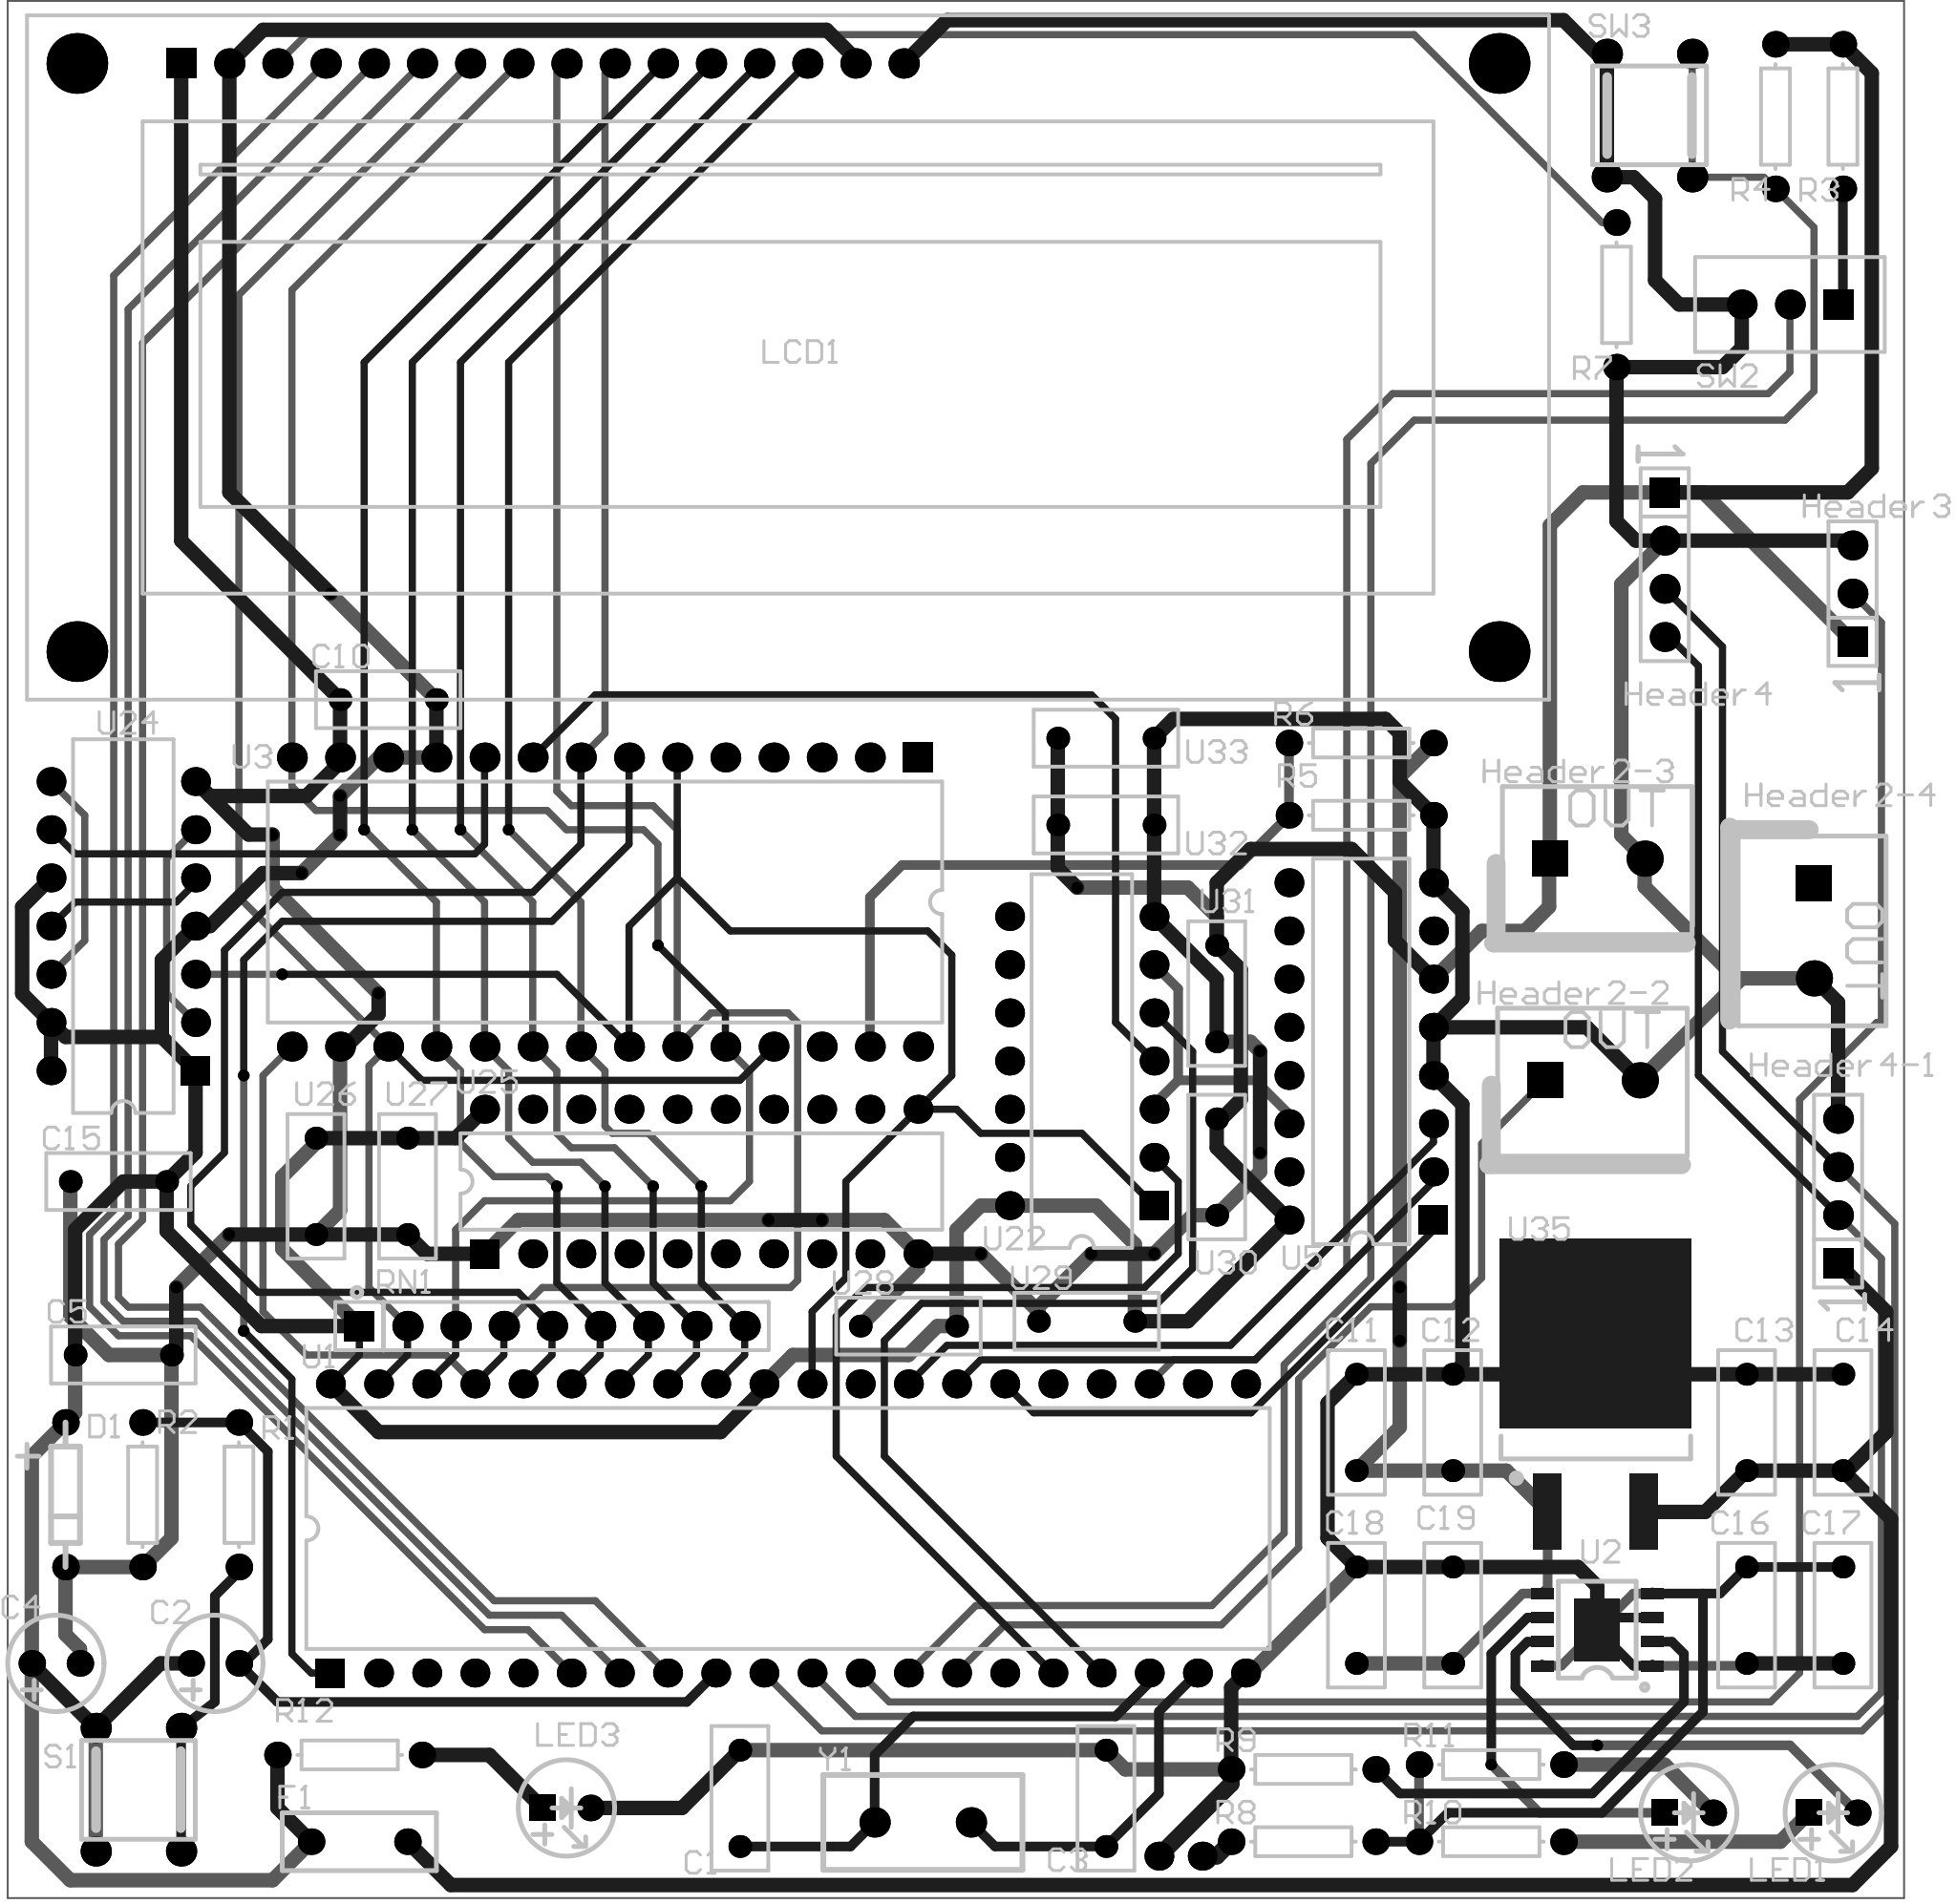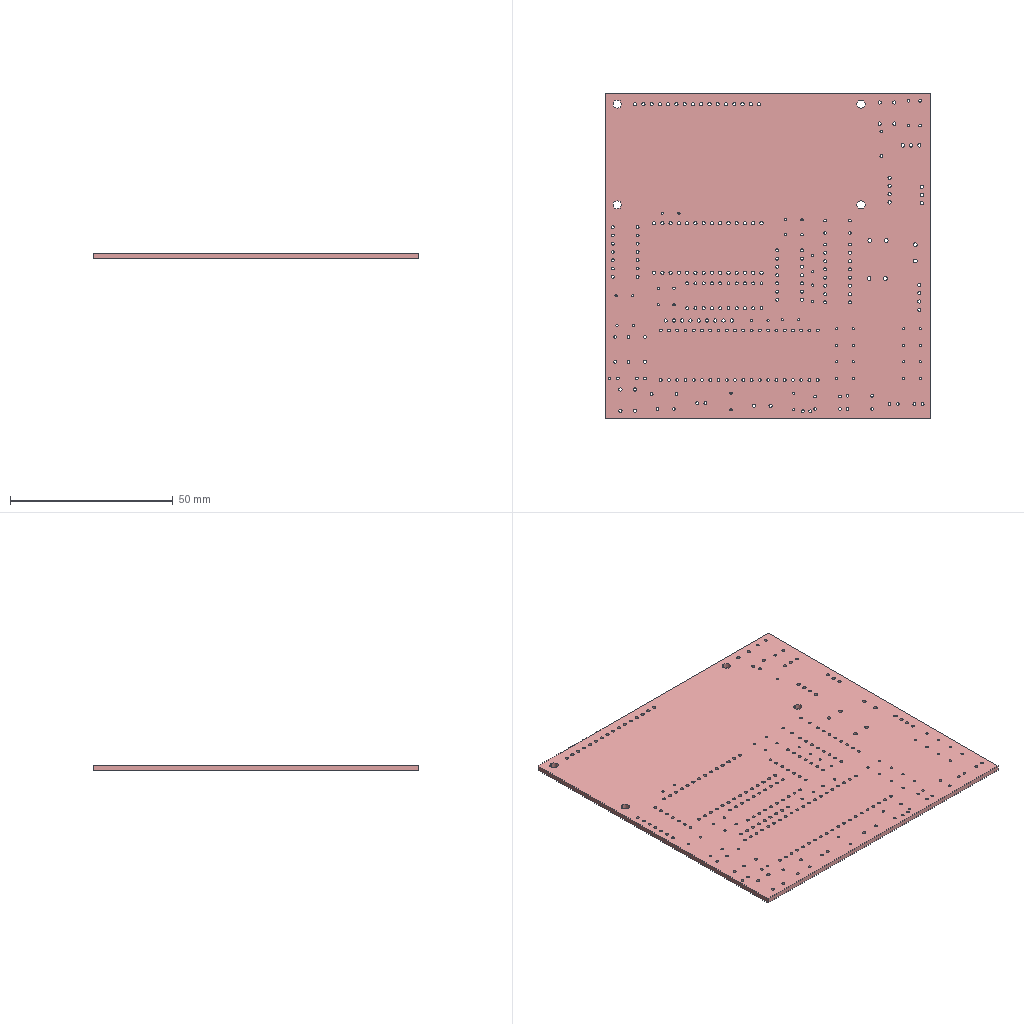Circuit board layout | Altium Designer | box 100 x 100 x 1.6 mm
Layer stack:
# Altium Designer layer stack of  (unit mm; dielectric type: 0 none, 1 core, 2 prepreg, 3 surface material)
index,name,kind,layer,copper_thickness_mm,dielectric_type,dielectric_thickness_mm,dielectric_material,dielectric_constant
0,Top Paste Mask Layer,other,,,,,,
1,Top Silkscreen Layer,other,,,,,,
2,Top Solder Mask Layer,dielectric,,,3,0.01,,3.3
3,Top Layer,copper,Top Layer,0.035,,,,
4,Dielectric1,dielectric,,,3,1.51,FR4,4.5
5,Bottom Layer,copper,Bottom Layer,0.035,,,,
6,Bottom Solder Mask Layer,dielectric,,,3,0.01,,3.3
7,Bottom Silkscreen Layer,other,,,,,,
8,Bottom Paste Mask Layer,other,,,,,,
# drill layer pairs: low layer,high layer
drill_pair,Top Layer,Bottom Layer
Part placement:
Designator,Comment,Layer,Footprint,Center-X(mm),Center-Y(mm),Rotation
U1,STC89C51RC-40I-PDIP40,TopLayer,DIP-40,117.348,95.682,0
Y1,11.059MHz,TopLayer,XTAL-2,124.455,80.189,0
C1,33pF,TopLayer,RAD-0.2,114.808,81.458,90
C3,33pF,TopLayer,RAD-0.2,134.112,81.458,90
C2,10uF,TopLayer,RB1-2,87.122,88.57,90
R1,200Ω,TopLayer,AXIAL-0.3,88.392,97.46,90
R2,10kΩ,TopLayer,AXIAL-0.3,83.312,97.46,270
S1,,TopLayer,RST,83.094,81.914,180
C5,100nF,TopLayer,RAD-0.2,82.296,104.826,0
C4,22uF,TopLayer,RB1-2,78.74,88.57,90
D1,1N5819,TopLayer,DIODE-3,79.248,97.46,180
F1,JK60-050,TopLayer,FUSE-2,94.742,79.172,0
U3,ADC0809CCV/NOPB,TopLayer,DIP-28,107.696,128.702,270
U5,74HC138D,653,TopLayer,DIP-16,147.574,120.828,180
U22,74HC02DRG,TopLayer,DIP-14,132.842,120.32,90
SW2,KH-SS12D01-G3-5.0,TopLayer,RT,170.18,160.198,90
Header4-1,PM254-1-04-W-8.5,TopLayer,CON4,172.72,113.462,90
U24,SN74HC74N,TopLayer,DIP-14,82.296,127.432,90
U25,74HC573D,653,TopLayer,DIP-20,112.776,113.97,0
U26,100nF,TopLayer,RAD-0.2,92.456,113.716,90
U27,100nF,TopLayer,RAD-0.2,97.282,113.716,90
U28,100nF,TopLayer,RAD-0.2,123.698,106.35,0
U29,100nF,TopLayer,RAD-0.2,133.096,106.604,0
U30,100nF,TopLayer,RAD-0.2,139.954,114.732,90
U31,100nF,TopLayer,RAD-0.2,139.954,123.876,90
U32,100nF,TopLayer,RAD-0.2,134.112,132.766,180
U33,100nF,TopLayer,RAD-0.2,134.112,137.338,180
RN1,4.7kΩ,TopLayer,RP,104.902,106.35,0
R3,1kΩ,TopLayer,AXIAL-0.3,172.974,170.104,90
C10,100nF,TopLayer,RAD-0.2,96.266,139.37,0
U35,LM7805S2/TR,TopLayer,TO-263-2_L10.0-W9.1-P5.08-LS15.2-BL,159.945,101.253,0
C11,100nF,TopLayer,RAD-0.2,147.32,101.27,270
C12,100nF,TopLayer,RAD-0.2,152.4,101.27,270
C13,10uF,TopLayer,RAD-0.2,167.894,101.27,270
C14,10uF,TopLayer,RAD-0.2,172.974,101.27,270
SW3,,TopLayer,RST,162.778,170.156,0
R4,10kΩ,TopLayer,AXIAL-0.3,169.418,170.104,90
LED1,204-10SYGD/S530-E3,TopLayer,LED1,172.466,80.696,90
LCD1,LCM1602K-NSW-BBW,TopLayer,LCD1602,117.348,157.404,0
Header4,PM254-1-04-W-8.5,TopLayer,CON4,163.576,146.482,270
R5,10kΩ,TopLayer,AXIAL-0.3,147.574,133.274,180
R6,10kΩ,TopLayer,AXIAL-0.3,147.574,137.084,0
C15,100nF,TopLayer,RAD-0.2,82.042,113.97,0
R7,3.5kΩ,TopLayer,AXIAL-0.3,161.036,160.706,90
Header2-2,XY-XHB2.54-2A21,TopLayer,CON2-5,159.766,119.304,0
Header3,PM254V-11-03-H85,TopLayer,CON3,173.482,144.958,0
Header2-3,XY-XHB2.54-2A21,TopLayer,CON2-5,160.02,130.988,0
Header2-4,XY-XHB2.54-2A21,TopLayer,CON2-5,171.45,127.178,270
C16,10uF,TopLayer,RAD-0.2,167.894,91.11,90
C17,100nF,TopLayer,RAD-0.2,172.974,91.11,90
LED2,333-2SYGD/S530-E2-L,TopLayer,LED1,164.846,80.696,90
R8,250mΩ,TopLayer,AXIAL-0.3,144.526,79.172,0
R9,1.2kΩ,TopLayer,AXIAL-0.3,144.526,82.982,0
R10,2kΩ,TopLayer,AXIAL-0.3,154.432,79.172,0
R11,2kΩ,TopLayer,AXIAL-0.3,154.432,83.236,0
C18,10uF,TopLayer,RAD-0.2,147.32,91.11,270
C19,100nF,TopLayer,RAD-0.2,152.4,91.11,270
R12,1kΩ,TopLayer,AXIAL-0.3,94.234,83.744,180
U2,TP4056-42-ESOP8,TopLayer,ESOP-8_L4.9-W3.9-P1.27-LS6.0-BL-EP,160.02,90.348,90
LED3,204-10SYGD/S530-E3,TopLayer,LED1,105.664,80.95,90
Pad and via stacks:
# Altium Designer via and pad stacks of  (unit mm). Each distinct definition once, with the count of objects using it.
# via: kind,start_layer,end_layer,hole_mm,diameter_mm,mode(0 simple;1 top-mid-bottom;2 full stack),diameter_per_layer,count,example_net
# pad: kind,layer,hole_mm,hole_type(0 round;1 square;2 slot),plating,top_size,top_shape(1 round;2 rect;3 octagon;9 rounded rect),mid_size,bottom_size,mode,footprint,size_per_layer,count,example
pad,Multi-Layer,0.9144,0,plated,1.524x1.524,1,1.524x1.524,1.524x1.524,0,,,2,41
pad,Multi-Layer,0.889,0,plated,1.524x1.524,1,1.524x1.524,1.524x1.524,0,DIP-40,,39,U1.18
pad,Multi-Layer,0.889,0,plated,1.524x1.524,2,1.524x1.524,1.524x1.524,0,DIP-40,,1,U1.1
pad,Multi-Layer,1,0,plated,1.6x1.6,1,1.6x1.6,1.6x1.6,0,XTAL-2,,2,Y1.1
pad,Multi-Layer,0.7,0,plated,1.2x1.2,1,1.2x1.2,1.2x1.2,0,RAD-0.2,,42,C1.2
pad,Multi-Layer,0.85,0,plated,1.4x1.4,1,1.4x1.4,1.4x1.4,0,RB1-2,,4,C2.2
pad,Multi-Layer,0.85,0,plated,1.4x1.4,1,1.4x1.4,1.4x1.4,0,AXIAL-0.3,,24,R1.2
pad,Multi-Layer,1,0,plated,1.6x1.6,1,1.6x1.6,1.6x1.6,0,RST,,8,S1.1
pad,Multi-Layer,0.85,0,plated,1.4x1.4,1,1.4x1.4,1.4x1.4,0,DIODE-3,,2,D1.2
pad,Multi-Layer,0.85,0,plated,1.4x1.4,1,1.4x1.4,1.4x1.4,0,FUSE-2,,2,F1.1
pad,Multi-Layer,1.016,0,plated,1.575x1.575,1,1.575x1.575,1.575x1.575,0,DIP-28,,27,U3.2
pad,Multi-Layer,1.016,0,plated,1.575x1.575,2,1.575x1.575,1.575x1.575,0,DIP-28,,1,U3.1
pad,Multi-Layer,0.889,0,plated,1.524x1.524,1,1.524x1.524,1.524x1.524,0,DIP-16,,15,U5.12
pad,Multi-Layer,0.889,0,plated,1.524x1.524,2,1.524x1.524,1.524x1.524,0,DIP-16,,1,U5.1
pad,Multi-Layer,0.889,0,plated,1.524x1.524,1,1.524x1.524,1.524x1.524,0,DIP-14,,26,U22.11
pad,Multi-Layer,0.889,0,plated,1.524x1.524,2,1.524x1.524,1.524x1.524,0,DIP-14,,2,U22.1
pad,Multi-Layer,1.016,0,plated,1.575x1.575,2,1.575x1.575,1.575x1.575,0,RT,,1,SW2.1
pad,Multi-Layer,1.016,0,plated,1.575x1.575,1,1.575x1.575,1.575x1.575,0,RT,,2,SW2.2
pad,Multi-Layer,1.016,0,plated,1.575x1.575,1,1.575x1.575,1.575x1.575,0,CON4,,6,Header4-1.4
pad,Multi-Layer,1.016,0,plated,1.575x1.575,2,1.575x1.575,1.575x1.575,0,CON4,,2,Header4-1.1
pad,Multi-Layer,0.889,0,plated,1.524x1.524,2,1.524x1.524,1.524x1.524,0,DIP-20,,1,U25.1
pad,Multi-Layer,0.889,0,plated,1.524x1.524,1,1.524x1.524,1.524x1.524,0,DIP-20,,19,U25.2
pad,Multi-Layer,1,0,plated,1.6x1.6,2,1.6x1.6,1.6x1.6,0,RP,,1,RN1.1
pad,Multi-Layer,1,0,plated,1.6x1.6,1,1.6x1.6,1.6x1.6,0,RP,,8,RN1.3
pad,Multi-Layer,0.85,0,plated,1.4x1.4,1,1.4x1.4,1.4x1.4,0,LED1,,3,LED1.2
pad,Multi-Layer,0.85,0,plated,1.4x1.4,2,1.4x1.4,1.4x1.4,0,LED1,,3,LED1.1
pad,Multi-Layer,1,0,plated,1.6x1.6,1,1.6x1.6,1.6x1.6,0,LCD1602,,15,LCD1.16
pad,Multi-Layer,1,0,plated,1.6x1.6,2,1.6x1.6,1.6x1.6,0,LCD1602,,1,LCD1.1
pad,Multi-Layer,2.5,2,plated,3.2x3.2,1,3.2x3.2,3.2x3.2,0,LCD1602,,4,LCD1.0
pad,Multi-Layer,1.194,0,plated,1.905x1.905,2,1.905x1.905,1.905x1.905,0,CON2-5,,3,Header2-2.1
pad,Multi-Layer,1.194,0,plated,1.905x1.905,1,1.905x1.905,1.905x1.905,0,CON2-5,,3,Header2-2.2
pad,Multi-Layer,1.016,0,plated,1.575x1.575,2,1.575x1.575,1.575x1.575,0,CON3,,1,Header3.1
pad,Multi-Layer,1.016,0,plated,1.575x1.575,1,1.575x1.575,1.575x1.575,0,CON3,,2,Header3.2
pad,Top Layer,0,0,plated,1.5x4,2,1.5x4,1.5x4,0,TO-263-2_L10.0-W9.1-P5.08-LS15.2-BL,,2,U35.1
pad,Top Layer,0,0,plated,10.1x10,2,10.1x10,10.1x10,0,TO-263-2_L10.0-W9.1-P5.08-LS15.2-BL,,1,U35.4
pad,Top Layer,0,0,plated,0.6x1.2,2,0.6x1.2,0.6x1.2,0,ESOP-8_L4.9-W3.9-P1.27-LS6.0-BL-EP,,8,U2.1
pad,Top Layer,0,0,plated,3.3x2.4,2,3.3x2.4,3.3x2.4,0,ESOP-8_L4.9-W3.9-P1.27-LS6.0-BL-EP,,1,U2.9
via,Top Layer,Bottom Layer,0.3048,0.61,0,,37,$1N30993
Design rules, without the lines most boards share:
# Altium Designer design rules of  (exported by Altium Designer, unit mm)
# columns: name | kind | enabled | priority | scope1 | scope2 | descriptor | typed fields (field=value)
otherClearance | 52 | enabled | 1 | All | All | Hole To Hole Clearance (Gap=11.8mil) (All),(All) | gap=0.2997